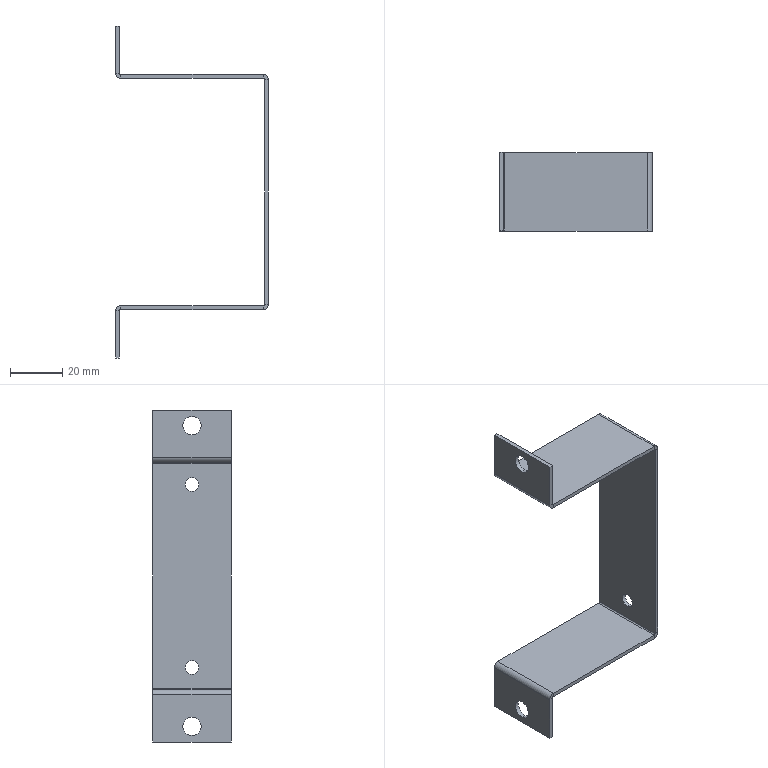Part | STEP file | 1 solid | 46 faces | box 58.5 x 30 x 127 mm | volume 10567 mm3 | plane 30 | cylinder 16 | commonest cylinder face diameters 1 x4 4 x4 5.3 x4 7 x4